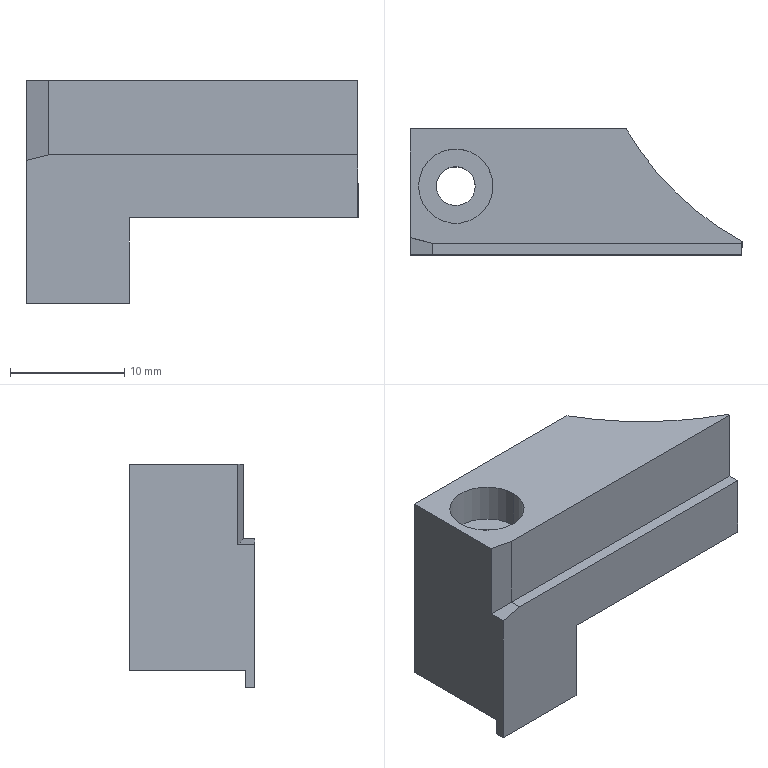Part | STEP file | 11-FG-B07111 | 1 solid | 20 faces | box 29 x 11 x 19.5 mm | volume 3288 mm3 | plane 15 | cylinder 5 | commonest cylinder face diameters 3.4 x2 6.5 x2 51 x1
STEP:
#1=CARTESIAN_POINT('',(-13.75,0.,14.6));
#2=VERTEX_POINT('',#1);
#3=CARTESIAN_POINT('',(-7.25,0.,14.6));
#4=VERTEX_POINT('',#3);
#5=CARTESIAN_POINT('',(-10.5,0.,14.6));
#6=DIRECTION('',(0.,0.,1.));
#7=DIRECTION('',(1.,0.,0.));
#8=AXIS2_PLACEMENT_3D('',#5,#6,#7);
#9=CIRCLE('',#8,3.25);
#10=EDGE_CURVE('',#2,#4,#9,.T.);
#11=ORIENTED_EDGE('',*,*,#10,.F.);
#12=CARTESIAN_POINT('',(-13.75,0.,18.));
#13=VERTEX_POINT('',#12);
#14=CARTESIAN_POINT('',(-13.75,0.,18.));
#15=DIRECTION('',(0.,0.,1.));
#16=VECTOR('',#15,1000.);
#17=LINE('',#14,#16);
#18=EDGE_CURVE('',#2,#13,#17,.T.);
#19=ORIENTED_EDGE('',*,*,#18,.T.);
#20=CARTESIAN_POINT('',(-7.25,0.,18.));
#21=VERTEX_POINT('',#20);
#22=CARTESIAN_POINT('',(-10.5,0.,18.));
#23=DIRECTION('',(0.,0.,1.));
#24=DIRECTION('',(1.,0.,0.));
#25=AXIS2_PLACEMENT_3D('',#22,#23,#24);
#26=CIRCLE('',#25,3.25);
#27=EDGE_CURVE('',#13,#21,#26,.T.);
#28=ORIENTED_EDGE('',*,*,#27,.T.);
#29=CARTESIAN_POINT('',(-7.25,0.,18.));
#30=DIRECTION('',(0.,0.,1.));
#31=VECTOR('',#30,1000.);
#32=LINE('',#29,#31);
#33=EDGE_CURVE('',#4,#21,#32,.T.);
#34=ORIENTED_EDGE('',*,*,#33,.F.);
#35=EDGE_LOOP('',(#11,#19,#28,#34));
#36=FACE_OUTER_BOUND('',#35,.T.);
#37=CARTESIAN_POINT('',(-10.5,0.,18.));
#38=DIRECTION('',(0.,0.,1.));
#39=DIRECTION('',(1.,0.,0.));
#40=AXIS2_PLACEMENT_3D('',#37,#38,#39);
#41=CYLINDRICAL_SURFACE('',#40,3.25);
#42=ADVANCED_FACE('',(#36),#41,.F.);
#43=CARTESIAN_POINT('',(-12.2,0.,0.));
#44=VERTEX_POINT('',#43);
#45=CARTESIAN_POINT('',(-8.8,0.,0.));
#46=VERTEX_POINT('',#45);
#47=CARTESIAN_POINT('',(-10.5,0.,0.));
#48=DIRECTION('',(0.,0.,1.));
#49=DIRECTION('',(1.,0.,0.));
#50=AXIS2_PLACEMENT_3D('',#47,#48,#49);
#51=CIRCLE('',#50,1.7);
#52=EDGE_CURVE('',#44,#46,#51,.T.);
#53=ORIENTED_EDGE('',*,*,#52,.F.);
#54=CARTESIAN_POINT('',(-12.2,0.,14.6));
#55=VERTEX_POINT('',#54);
#56=CARTESIAN_POINT('',(-12.2,0.,18.));
#57=DIRECTION('',(0.,0.,1.));
#58=VECTOR('',#57,1000.);
#59=LINE('',#56,#58);
#60=EDGE_CURVE('',#44,#55,#59,.T.);
#61=ORIENTED_EDGE('',*,*,#60,.T.);
#62=CARTESIAN_POINT('',(-8.8,0.,14.6));
#63=VERTEX_POINT('',#62);
#64=CARTESIAN_POINT('',(-10.5,0.,14.6));
#65=DIRECTION('',(0.,0.,1.));
#66=DIRECTION('',(1.,0.,0.));
#67=AXIS2_PLACEMENT_3D('',#64,#65,#66);
#68=CIRCLE('',#67,1.7);
#69=EDGE_CURVE('',#55,#63,#68,.T.);
#70=ORIENTED_EDGE('',*,*,#69,.T.);
#71=CARTESIAN_POINT('',(-8.8,0.,18.));
#72=DIRECTION('',(0.,0.,1.));
#73=VECTOR('',#72,1000.);
#74=LINE('',#71,#73);
#75=EDGE_CURVE('',#46,#63,#74,.T.);
#76=ORIENTED_EDGE('',*,*,#75,.F.);
#77=EDGE_LOOP('',(#53,#61,#70,#76));
#78=FACE_OUTER_BOUND('',#77,.T.);
#79=CARTESIAN_POINT('',(-10.5,0.,18.));
#80=DIRECTION('',(0.,0.,1.));
#81=DIRECTION('',(1.,0.,0.));
#82=AXIS2_PLACEMENT_3D('',#79,#80,#81);
#83=CYLINDRICAL_SURFACE('',#82,1.7);
#84=ADVANCED_FACE('',(#78),#83,.F.);
#85=CARTESIAN_POINT('',(-10.5,0.,0.));
#86=DIRECTION('',(0.,0.,1.));
#87=DIRECTION('',(1.,0.,0.));
#88=AXIS2_PLACEMENT_3D('',#85,#86,#87);
#89=CIRCLE('',#88,1.7);
#90=EDGE_CURVE('',#46,#44,#89,.T.);
#91=ORIENTED_EDGE('',*,*,#90,.T.);
#92=ORIENTED_EDGE('',*,*,#52,.T.);
#93=EDGE_LOOP('',(#91,#92));
#94=FACE_BOUND('',#93,.T.);
#95=CARTESIAN_POINT('',(-14.5,-5.2,0.));
#96=VERTEX_POINT('',#95);
#97=CARTESIAN_POINT('',(-5.5,-5.2,0.));
#98=VERTEX_POINT('',#97);
#99=CARTESIAN_POINT('',(-14.5,-5.2,0.));
#100=DIRECTION('',(1.,0.,0.));
#101=VECTOR('',#100,1000.);
#102=LINE('',#99,#101);
#103=EDGE_CURVE('',#96,#98,#102,.T.);
#104=ORIENTED_EDGE('',*,*,#103,.F.);
#105=CARTESIAN_POINT('',(-14.5,5.,0.));
#106=VERTEX_POINT('',#105);
#107=CARTESIAN_POINT('',(-14.5,-5.,0.));
#108=DIRECTION('',(0.,-1.,0.));
#109=VECTOR('',#108,1000.);
#110=LINE('',#107,#109);
#111=EDGE_CURVE('',#106,#96,#110,.T.);
#112=ORIENTED_EDGE('',*,*,#111,.F.);
#113=CARTESIAN_POINT('',(-5.5,5.,0.));
#114=VERTEX_POINT('',#113);
#115=CARTESIAN_POINT('',(14.5,5.,0.));
#116=DIRECTION('',(-1.,0.,0.));
#117=VECTOR('',#116,1000.);
#118=LINE('',#115,#117);
#119=EDGE_CURVE('',#114,#106,#118,.T.);
#120=ORIENTED_EDGE('',*,*,#119,.F.);
#121=CARTESIAN_POINT('',(-5.5,-5.,0.));
#122=DIRECTION('',(0.,1.,0.));
#123=VECTOR('',#122,1000.);
#124=LINE('',#121,#123);
#125=EDGE_CURVE('',#98,#114,#124,.T.);
#126=ORIENTED_EDGE('',*,*,#125,.F.);
#127=EDGE_LOOP('',(#104,#112,#120,#126));
#128=FACE_OUTER_BOUND('',#127,.T.);
#129=CARTESIAN_POINT('',(0.,0.,0.));
#130=DIRECTION('',(0.,0.,1.));
#131=DIRECTION('',(1.,0.,0.));
#132=AXIS2_PLACEMENT_3D('',#129,#130,#131);
#133=PLANE('',#132);
#134=ADVANCED_FACE('',(#94,#128),#133,.F.);
#135=CARTESIAN_POINT('',(-12.5,-5.,18.));
#136=VERTEX_POINT('',#135);
#137=CARTESIAN_POINT('',(14.5,-5.,18.));
#138=VERTEX_POINT('',#137);
#139=CARTESIAN_POINT('',(14.5,-5.,18.));
#140=DIRECTION('',(1.,0.,0.));
#141=VECTOR('',#140,1000.);
#142=LINE('',#139,#141);
#143=EDGE_CURVE('',#136,#138,#142,.T.);
#144=ORIENTED_EDGE('',*,*,#143,.F.);
#145=CARTESIAN_POINT('',(-12.5,-5.,11.5));
#146=VERTEX_POINT('',#145);
#147=CARTESIAN_POINT('',(-12.5,-5.,18.));
#148=DIRECTION('',(0.,0.,-1.));
#149=VECTOR('',#148,1000.);
#150=LINE('',#147,#149);
#151=EDGE_CURVE('',#136,#146,#150,.T.);
#152=ORIENTED_EDGE('',*,*,#151,.T.);
#153=CARTESIAN_POINT('',(14.5,-5.,11.5));
#154=VERTEX_POINT('',#153);
#155=CARTESIAN_POINT('',(-14.5,-5.,11.5));
#156=DIRECTION('',(-1.,0.,0.));
#157=VECTOR('',#156,1000.);
#158=LINE('',#155,#157);
#159=EDGE_CURVE('',#154,#146,#158,.T.);
#160=ORIENTED_EDGE('',*,*,#159,.F.);
#161=CARTESIAN_POINT('',(14.5,-5.,18.));
#162=DIRECTION('',(0.,0.,-1.));
#163=VECTOR('',#162,1000.);
#164=LINE('',#161,#163);
#165=EDGE_CURVE('',#138,#154,#164,.T.);
#166=ORIENTED_EDGE('',*,*,#165,.F.);
#167=EDGE_LOOP('',(#144,#152,#160,#166));
#168=FACE_OUTER_BOUND('',#167,.T.);
#169=CARTESIAN_POINT('',(14.5,-5.,18.));
#170=DIRECTION('',(0.,1.,0.));
#171=DIRECTION('',(-1.,0.,0.));
#172=AXIS2_PLACEMENT_3D('',#169,#170,#171);
#173=PLANE('',#172);
#174=ADVANCED_FACE('',(#168),#173,.F.);
#175=CARTESIAN_POINT('',(-14.5,-6.,11.));
#176=VERTEX_POINT('',#175);
#177=CARTESIAN_POINT('',(-14.5,-6.,-1.5));
#178=VERTEX_POINT('',#177);
#179=CARTESIAN_POINT('',(-14.5,-6.,0.));
#180=DIRECTION('',(0.,0.,-1.));
#181=VECTOR('',#180,1000.);
#182=LINE('',#179,#181);
#183=EDGE_CURVE('',#176,#178,#182,.T.);
#184=ORIENTED_EDGE('',*,*,#183,.F.);
#185=CARTESIAN_POINT('',(-14.5,-4.5,11.));
#186=VERTEX_POINT('',#185);
#187=CARTESIAN_POINT('',(-14.5,-5.,11.));
#188=DIRECTION('',(0.,1.,0.));
#189=VECTOR('',#188,1000.);
#190=LINE('',#187,#189);
#191=EDGE_CURVE('',#176,#186,#190,.T.);
#192=ORIENTED_EDGE('',*,*,#191,.T.);
#193=CARTESIAN_POINT('',(-14.5,-4.5,18.));
#194=VERTEX_POINT('',#193);
#195=CARTESIAN_POINT('',(-14.5,-4.5,18.));
#196=DIRECTION('',(0.,0.,1.));
#197=VECTOR('',#196,1000.);
#198=LINE('',#195,#197);
#199=EDGE_CURVE('',#186,#194,#198,.T.);
#200=ORIENTED_EDGE('',*,*,#199,.T.);
#201=CARTESIAN_POINT('',(-14.5,5.,18.));
#202=VERTEX_POINT('',#201);
#203=CARTESIAN_POINT('',(-14.5,-5.,18.));
#204=DIRECTION('',(0.,-1.,0.));
#205=VECTOR('',#204,1000.);
#206=LINE('',#203,#205);
#207=EDGE_CURVE('',#202,#194,#206,.T.);
#208=ORIENTED_EDGE('',*,*,#207,.F.);
#209=CARTESIAN_POINT('',(-14.5,5.,18.));
#210=DIRECTION('',(0.,0.,-1.));
#211=VECTOR('',#210,1000.);
#212=LINE('',#209,#211);
#213=EDGE_CURVE('',#202,#106,#212,.T.);
#214=ORIENTED_EDGE('',*,*,#213,.T.);
#215=ORIENTED_EDGE('',*,*,#111,.T.);
#216=CARTESIAN_POINT('',(-14.5,-5.2,-1.5));
#217=VERTEX_POINT('',#216);
#218=CARTESIAN_POINT('',(-14.5,-5.2,-1.5));
#219=DIRECTION('',(0.,0.,1.));
#220=VECTOR('',#219,1000.);
#221=LINE('',#218,#220);
#222=EDGE_CURVE('',#217,#96,#221,.T.);
#223=ORIENTED_EDGE('',*,*,#222,.F.);
#224=CARTESIAN_POINT('',(-14.5,-6.,-1.5));
#225=DIRECTION('',(0.,1.,0.));
#226=VECTOR('',#225,1000.);
#227=LINE('',#224,#226);
#228=EDGE_CURVE('',#178,#217,#227,.T.);
#229=ORIENTED_EDGE('',*,*,#228,.F.);
#230=EDGE_LOOP('',(#184,#192,#200,#208,#214,#215,#223,#229));
#231=FACE_OUTER_BOUND('',#230,.T.);
#232=CARTESIAN_POINT('',(-14.5,-5.,18.));
#233=DIRECTION('',(1.,0.,0.));
#234=DIRECTION('',(0.,0.,-1.));
#235=AXIS2_PLACEMENT_3D('',#232,#233,#234);
#236=PLANE('',#235);
#237=ADVANCED_FACE('',(#231),#236,.F.);
#238=CARTESIAN_POINT('',(14.5,-6.,6.));
#239=VERTEX_POINT('',#238);
#240=CARTESIAN_POINT('',(14.5,-4.8,6.));
#241=VERTEX_POINT('',#240);
#242=CARTESIAN_POINT('',(14.5,-5.,6.));
#243=DIRECTION('',(0.,1.,0.));
#244=VECTOR('',#243,1000.);
#245=LINE('',#242,#244);
#246=EDGE_CURVE('',#239,#241,#245,.T.);
#247=ORIENTED_EDGE('',*,*,#246,.T.);
#248=CARTESIAN_POINT('',(14.5,-4.8,18.));
#249=VERTEX_POINT('',#248);
#250=CARTESIAN_POINT('',(14.5,-4.8,0.));
#251=DIRECTION('',(0.,0.,1.));
#252=VECTOR('',#251,1000.);
#253=LINE('',#250,#252);
#254=EDGE_CURVE('',#241,#249,#253,.T.);
#255=ORIENTED_EDGE('',*,*,#254,.T.);
#256=CARTESIAN_POINT('',(14.5,-5.,18.));
#257=DIRECTION('',(0.,1.,0.));
#258=VECTOR('',#257,1000.);
#259=LINE('',#256,#258);
#260=EDGE_CURVE('',#138,#249,#259,.T.);
#261=ORIENTED_EDGE('',*,*,#260,.F.);
#262=ORIENTED_EDGE('',*,*,#165,.T.);
#263=CARTESIAN_POINT('',(14.5,-6.,11.5));
#264=VERTEX_POINT('',#263);
#265=CARTESIAN_POINT('',(14.5,-6.,11.5));
#266=DIRECTION('',(0.,1.,0.));
#267=VECTOR('',#266,1000.);
#268=LINE('',#265,#267);
#269=EDGE_CURVE('',#264,#154,#268,.T.);
#270=ORIENTED_EDGE('',*,*,#269,.F.);
#271=CARTESIAN_POINT('',(14.5,-6.,6.));
#272=DIRECTION('',(0.,0.,1.));
#273=VECTOR('',#272,1000.);
#274=LINE('',#271,#273);
#275=EDGE_CURVE('',#239,#264,#274,.T.);
#276=ORIENTED_EDGE('',*,*,#275,.F.);
#277=EDGE_LOOP('',(#247,#255,#261,#262,#270,#276));
#278=FACE_OUTER_BOUND('',#277,.T.);
#279=CARTESIAN_POINT('',(14.5,-5.,18.));
#280=DIRECTION('',(-1.,0.,0.));
#281=DIRECTION('',(0.,0.,1.));
#282=AXIS2_PLACEMENT_3D('',#279,#280,#281);
#283=PLANE('',#282);
#284=ADVANCED_FACE('',(#278),#283,.F.);
#285=CARTESIAN_POINT('',(4.388,5.,18.));
#286=VERTEX_POINT('',#285);
#287=CARTESIAN_POINT('',(14.5,5.,18.));
#288=DIRECTION('',(-1.,0.,0.));
#289=VECTOR('',#288,1000.);
#290=LINE('',#287,#289);
#291=EDGE_CURVE('',#286,#202,#290,.T.);
#292=ORIENTED_EDGE('',*,*,#291,.F.);
#293=CARTESIAN_POINT('',(4.388,5.,6.));
#294=VERTEX_POINT('',#293);
#295=CARTESIAN_POINT('',(4.388,5.,0.));
#296=DIRECTION('',(0.,0.,-1.));
#297=VECTOR('',#296,1000.);
#298=LINE('',#295,#297);
#299=EDGE_CURVE('',#286,#294,#298,.T.);
#300=ORIENTED_EDGE('',*,*,#299,.T.);
#301=CARTESIAN_POINT('',(-5.5,5.,6.));
#302=VERTEX_POINT('',#301);
#303=CARTESIAN_POINT('',(-5.5,5.,6.));
#304=DIRECTION('',(1.,0.,0.));
#305=VECTOR('',#304,1000.);
#306=LINE('',#303,#305);
#307=EDGE_CURVE('',#302,#294,#306,.T.);
#308=ORIENTED_EDGE('',*,*,#307,.F.);
#309=CARTESIAN_POINT('',(-5.5,5.,0.));
#310=DIRECTION('',(0.,0.,1.));
#311=VECTOR('',#310,1000.);
#312=LINE('',#309,#311);
#313=EDGE_CURVE('',#114,#302,#312,.T.);
#314=ORIENTED_EDGE('',*,*,#313,.F.);
#315=ORIENTED_EDGE('',*,*,#119,.T.);
#316=ORIENTED_EDGE('',*,*,#213,.F.);
#317=EDGE_LOOP('',(#292,#300,#308,#314,#315,#316));
#318=FACE_OUTER_BOUND('',#317,.T.);
#319=CARTESIAN_POINT('',(14.5,5.,18.));
#320=DIRECTION('',(0.,-1.,0.));
#321=DIRECTION('',(1.,0.,0.));
#322=AXIS2_PLACEMENT_3D('',#319,#320,#321);
#323=PLANE('',#322);
#324=ADVANCED_FACE('',(#318),#323,.F.);
#325=ORIENTED_EDGE('',*,*,#207,.T.);
#326=CARTESIAN_POINT('',(-1.912,-7.647,18.));
#327=DIRECTION('',(0.9701,-0.2425,0.));
#328=VECTOR('',#327,1000.);
#329=LINE('',#326,#328);
#330=EDGE_CURVE('',#194,#136,#329,.T.);
#331=ORIENTED_EDGE('',*,*,#330,.T.);
#332=ORIENTED_EDGE('',*,*,#143,.T.);
#333=ORIENTED_EDGE('',*,*,#260,.T.);
#334=CARTESIAN_POINT('',(26.5,17.7,18.));
#335=DIRECTION('',(0.,0.,1.));
#336=DIRECTION('',(1.,0.,0.));
#337=AXIS2_PLACEMENT_3D('',#334,#335,#336);
#338=CIRCLE('',#337,25.5);
#339=EDGE_CURVE('',#286,#249,#338,.T.);
#340=ORIENTED_EDGE('',*,*,#339,.F.);
#341=ORIENTED_EDGE('',*,*,#291,.T.);
#342=EDGE_LOOP('',(#325,#331,#332,#333,#340,#341));
#343=FACE_OUTER_BOUND('',#342,.T.);
#344=CARTESIAN_POINT('',(-10.5,0.,18.));
#345=DIRECTION('',(0.,0.,1.));
#346=DIRECTION('',(1.,0.,0.));
#347=AXIS2_PLACEMENT_3D('',#344,#345,#346);
#348=CIRCLE('',#347,3.25);
#349=EDGE_CURVE('',#21,#13,#348,.T.);
#350=ORIENTED_EDGE('',*,*,#349,.F.);
#351=ORIENTED_EDGE('',*,*,#27,.F.);
#352=EDGE_LOOP('',(#350,#351));
#353=FACE_BOUND('',#352,.T.);
#354=CARTESIAN_POINT('',(0.,0.,18.));
#355=DIRECTION('',(0.,0.,1.));
#356=DIRECTION('',(1.,0.,0.));
#357=AXIS2_PLACEMENT_3D('',#354,#355,#356);
#358=PLANE('',#357);
#359=ADVANCED_FACE('',(#343,#353),#358,.T.);
#360=ORIENTED_EDGE('',*,*,#313,.T.);
#361=CARTESIAN_POINT('',(-5.5,-6.,6.));
#362=VERTEX_POINT('',#361);
#363=CARTESIAN_POINT('',(-5.5,-5.,6.));
#364=DIRECTION('',(0.,1.,0.));
#365=VECTOR('',#364,1000.);
#366=LINE('',#363,#365);
#367=EDGE_CURVE('',#362,#302,#366,.T.);
#368=ORIENTED_EDGE('',*,*,#367,.F.);
#369=CARTESIAN_POINT('',(-5.5,-6.,-1.5));
#370=VERTEX_POINT('',#369);
#371=CARTESIAN_POINT('',(-5.5,-6.,6.));
#372=DIRECTION('',(0.,0.,1.));
#373=VECTOR('',#372,1000.);
#374=LINE('',#371,#373);
#375=EDGE_CURVE('',#370,#362,#374,.T.);
#376=ORIENTED_EDGE('',*,*,#375,.F.);
#377=CARTESIAN_POINT('',(-5.5,-5.2,-1.5));
#378=VERTEX_POINT('',#377);
#379=CARTESIAN_POINT('',(-5.5,-6.,-1.5));
#380=DIRECTION('',(0.,-1.,0.));
#381=VECTOR('',#380,1000.);
#382=LINE('',#379,#381);
#383=EDGE_CURVE('',#378,#370,#382,.T.);
#384=ORIENTED_EDGE('',*,*,#383,.F.);
#385=CARTESIAN_POINT('',(-5.5,-5.2,-1.5));
#386=DIRECTION('',(0.,0.,1.));
#387=VECTOR('',#386,1000.);
#388=LINE('',#385,#387);
#389=EDGE_CURVE('',#378,#98,#388,.T.);
#390=ORIENTED_EDGE('',*,*,#389,.T.);
#391=ORIENTED_EDGE('',*,*,#125,.T.);
#392=EDGE_LOOP('',(#360,#368,#376,#384,#390,#391));
#393=FACE_OUTER_BOUND('',#392,.T.);
#394=CARTESIAN_POINT('',(-5.5,-5.,0.));
#395=DIRECTION('',(-1.,0.,0.));
#396=DIRECTION('',(0.,-1.,0.));
#397=AXIS2_PLACEMENT_3D('',#394,#395,#396);
#398=PLANE('',#397);
#399=ADVANCED_FACE('',(#393),#398,.F.);
#400=ORIENTED_EDGE('',*,*,#307,.T.);
#401=CARTESIAN_POINT('',(26.5,17.7,6.));
#402=DIRECTION('',(0.,0.,1.));
#403=DIRECTION('',(1.,0.,0.));
#404=AXIS2_PLACEMENT_3D('',#401,#402,#403);
#405=CIRCLE('',#404,25.5);
#406=EDGE_CURVE('',#294,#241,#405,.T.);
#407=ORIENTED_EDGE('',*,*,#406,.T.);
#408=ORIENTED_EDGE('',*,*,#246,.F.);
#409=CARTESIAN_POINT('',(-5.5,-6.,6.));
#410=DIRECTION('',(1.,0.,0.));
#411=VECTOR('',#410,1000.);
#412=LINE('',#409,#411);
#413=EDGE_CURVE('',#362,#239,#412,.T.);
#414=ORIENTED_EDGE('',*,*,#413,.F.);
#415=ORIENTED_EDGE('',*,*,#367,.T.);
#416=EDGE_LOOP('',(#400,#407,#408,#414,#415));
#417=FACE_OUTER_BOUND('',#416,.T.);
#418=CARTESIAN_POINT('',(-5.5,-5.,6.));
#419=DIRECTION('',(0.,0.,1.));
#420=DIRECTION('',(1.,0.,0.));
#421=AXIS2_PLACEMENT_3D('',#418,#419,#420);
#422=PLANE('',#421);
#423=ADVANCED_FACE('',(#417),#422,.F.);
#424=ORIENTED_EDGE('',*,*,#60,.F.);
#425=ORIENTED_EDGE('',*,*,#90,.F.);
#426=ORIENTED_EDGE('',*,*,#75,.T.);
#427=CARTESIAN_POINT('',(-10.5,0.,14.6));
#428=DIRECTION('',(0.,0.,1.));
#429=DIRECTION('',(1.,0.,0.));
#430=AXIS2_PLACEMENT_3D('',#427,#428,#429);
#431=CIRCLE('',#430,1.7);
#432=EDGE_CURVE('',#63,#55,#431,.T.);
#433=ORIENTED_EDGE('',*,*,#432,.T.);
#434=EDGE_LOOP('',(#424,#425,#426,#433));
#435=FACE_OUTER_BOUND('',#434,.T.);
#436=CARTESIAN_POINT('',(-10.5,0.,18.));
#437=DIRECTION('',(0.,0.,1.));
#438=DIRECTION('',(1.,0.,0.));
#439=AXIS2_PLACEMENT_3D('',#436,#437,#438);
#440=CYLINDRICAL_SURFACE('',#439,1.7);
#441=ADVANCED_FACE('',(#435),#440,.F.);
#442=ORIENTED_EDGE('',*,*,#432,.F.);
#443=ORIENTED_EDGE('',*,*,#69,.F.);
#444=EDGE_LOOP('',(#442,#443));
#445=FACE_BOUND('',#444,.T.);
#446=CARTESIAN_POINT('',(-10.5,0.,14.6));
#447=DIRECTION('',(0.,0.,1.));
#448=DIRECTION('',(1.,0.,0.));
#449=AXIS2_PLACEMENT_3D('',#446,#447,#448);
#450=CIRCLE('',#449,3.25);
#451=EDGE_CURVE('',#4,#2,#450,.T.);
#452=ORIENTED_EDGE('',*,*,#451,.T.);
#453=ORIENTED_EDGE('',*,*,#10,.T.);
#454=EDGE_LOOP('',(#452,#453));
#455=FACE_OUTER_BOUND('',#454,.T.);
#456=CARTESIAN_POINT('',(-8.8,0.,14.6));
#457=DIRECTION('',(0.,0.,-1.));
#458=DIRECTION('',(-1.,0.,0.));
#459=AXIS2_PLACEMENT_3D('',#456,#457,#458);
#460=PLANE('',#459);
#461=ADVANCED_FACE('',(#445,#455),#460,.F.);
#462=ORIENTED_EDGE('',*,*,#18,.F.);
#463=ORIENTED_EDGE('',*,*,#451,.F.);
#464=ORIENTED_EDGE('',*,*,#33,.T.);
#465=ORIENTED_EDGE('',*,*,#349,.T.);
#466=EDGE_LOOP('',(#462,#463,#464,#465));
#467=FACE_OUTER_BOUND('',#466,.T.);
#468=CARTESIAN_POINT('',(-10.5,0.,18.));
#469=DIRECTION('',(0.,0.,1.));
#470=DIRECTION('',(1.,0.,0.));
#471=AXIS2_PLACEMENT_3D('',#468,#469,#470);
#472=CYLINDRICAL_SURFACE('',#471,3.25);
#473=ADVANCED_FACE('',(#467),#472,.F.);
#474=ORIENTED_EDGE('',*,*,#406,.F.);
#475=ORIENTED_EDGE('',*,*,#299,.F.);
#476=ORIENTED_EDGE('',*,*,#339,.T.);
#477=ORIENTED_EDGE('',*,*,#254,.F.);
#478=EDGE_LOOP('',(#474,#475,#476,#477));
#479=FACE_OUTER_BOUND('',#478,.T.);
#480=CARTESIAN_POINT('',(26.5,17.7,0.));
#481=DIRECTION('',(0.,0.,1.));
#482=DIRECTION('',(1.,0.,0.));
#483=AXIS2_PLACEMENT_3D('',#480,#481,#482);
#484=CYLINDRICAL_SURFACE('',#483,25.5);
#485=ADVANCED_FACE('',(#479),#484,.F.);
#486=ORIENTED_EDGE('',*,*,#159,.T.);
#487=CARTESIAN_POINT('',(-12.5,-6.,11.5));
#488=VERTEX_POINT('',#487);
#489=CARTESIAN_POINT('',(-12.5,-6.,11.5));
#490=DIRECTION('',(0.,-1.,0.));
#491=VECTOR('',#490,1000.);
#492=LINE('',#489,#491);
#493=EDGE_CURVE('',#146,#488,#492,.T.);
#494=ORIENTED_EDGE('',*,*,#493,.T.);
#495=CARTESIAN_POINT('',(-14.5,-6.,11.5));
#496=DIRECTION('',(-1.,0.,0.));
#497=VECTOR('',#496,1000.);
#498=LINE('',#495,#497);
#499=EDGE_CURVE('',#264,#488,#498,.T.);
#500=ORIENTED_EDGE('',*,*,#499,.F.);
#501=ORIENTED_EDGE('',*,*,#269,.T.);
#502=EDGE_LOOP('',(#486,#494,#500,#501));
#503=FACE_OUTER_BOUND('',#502,.T.);
#504=CARTESIAN_POINT('',(-14.5,-6.,11.5));
#505=DIRECTION('',(0.,0.,-1.));
#506=DIRECTION('',(-1.,0.,0.));
#507=AXIS2_PLACEMENT_3D('',#504,#505,#506);
#508=PLANE('',#507);
#509=ADVANCED_FACE('',(#503),#508,.F.);
#510=ORIENTED_EDGE('',*,*,#499,.T.);
#511=CARTESIAN_POINT('',(-14.5,-6.,11.));
#512=DIRECTION('',(-0.9701,0.,-0.2425));
#513=VECTOR('',#512,1000.);
#514=LINE('',#511,#513);
#515=EDGE_CURVE('',#488,#176,#514,.T.);
#516=ORIENTED_EDGE('',*,*,#515,.T.);
#517=ORIENTED_EDGE('',*,*,#183,.T.);
#518=CARTESIAN_POINT('',(-14.5,-6.,-1.5));
#519=DIRECTION('',(-1.,0.,0.));
#520=VECTOR('',#519,1000.);
#521=LINE('',#518,#520);
#522=EDGE_CURVE('',#370,#178,#521,.T.);
#523=ORIENTED_EDGE('',*,*,#522,.F.);
#524=ORIENTED_EDGE('',*,*,#375,.T.);
#525=ORIENTED_EDGE('',*,*,#413,.T.);
#526=ORIENTED_EDGE('',*,*,#275,.T.);
#527=EDGE_LOOP('',(#510,#516,#517,#523,#524,#525,#526));
#528=FACE_OUTER_BOUND('',#527,.T.);
#529=CARTESIAN_POINT('',(0.,-6.,0.));
#530=DIRECTION('',(0.,1.,0.));
#531=DIRECTION('',(-1.,0.,0.));
#532=AXIS2_PLACEMENT_3D('',#529,#530,#531);
#533=PLANE('',#532);
#534=ADVANCED_FACE('',(#528),#533,.F.);
#535=ORIENTED_EDGE('',*,*,#330,.F.);
#536=ORIENTED_EDGE('',*,*,#199,.F.);
#537=CARTESIAN_POINT('',(-14.389,-4.528,11.028));
#538=DIRECTION('',(-0.9428,0.2357,-0.2357));
#539=VECTOR('',#538,1000.);
#540=LINE('',#537,#539);
#541=EDGE_CURVE('',#146,#186,#540,.T.);
#542=ORIENTED_EDGE('',*,*,#541,.F.);
#543=ORIENTED_EDGE('',*,*,#151,.F.);
#544=EDGE_LOOP('',(#535,#536,#542,#543));
#545=FACE_OUTER_BOUND('',#544,.T.);
#546=CARTESIAN_POINT('',(-12.5,-5.,18.));
#547=DIRECTION('',(0.2425,0.9701,0.));
#548=DIRECTION('',(0.,0.,-1.));
#549=AXIS2_PLACEMENT_3D('',#546,#547,#548);
#550=PLANE('',#549);
#551=ADVANCED_FACE('',(#545),#550,.F.);
#552=ORIENTED_EDGE('',*,*,#515,.F.);
#553=ORIENTED_EDGE('',*,*,#493,.F.);
#554=ORIENTED_EDGE('',*,*,#541,.T.);
#555=ORIENTED_EDGE('',*,*,#191,.F.);
#556=EDGE_LOOP('',(#552,#553,#554,#555));
#557=FACE_OUTER_BOUND('',#556,.T.);
#558=CARTESIAN_POINT('',(-14.5,-5.,11.));
#559=DIRECTION('',(0.2425,0.,-0.9701));
#560=DIRECTION('',(0.,1.,0.));
#561=AXIS2_PLACEMENT_3D('',#558,#559,#560);
#562=PLANE('',#561);
#563=ADVANCED_FACE('',(#557),#562,.F.);
#564=ORIENTED_EDGE('',*,*,#103,.T.);
#565=ORIENTED_EDGE('',*,*,#389,.F.);
#566=CARTESIAN_POINT('',(-14.5,-5.2,-1.5));
#567=DIRECTION('',(1.,0.,0.));
#568=VECTOR('',#567,1000.);
#569=LINE('',#566,#568);
#570=EDGE_CURVE('',#217,#378,#569,.T.);
#571=ORIENTED_EDGE('',*,*,#570,.F.);
#572=ORIENTED_EDGE('',*,*,#222,.T.);
#573=EDGE_LOOP('',(#564,#565,#571,#572));
#574=FACE_OUTER_BOUND('',#573,.T.);
#575=CARTESIAN_POINT('',(-14.5,-5.2,-1.5));
#576=DIRECTION('',(0.,-1.,0.));
#577=DIRECTION('',(0.,0.,-1.));
#578=AXIS2_PLACEMENT_3D('',#575,#576,#577);
#579=PLANE('',#578);
#580=ADVANCED_FACE('',(#574),#579,.F.);
#581=ORIENTED_EDGE('',*,*,#228,.T.);
#582=ORIENTED_EDGE('',*,*,#570,.T.);
#583=ORIENTED_EDGE('',*,*,#383,.T.);
#584=ORIENTED_EDGE('',*,*,#522,.T.);
#585=EDGE_LOOP('',(#581,#582,#583,#584));
#586=FACE_OUTER_BOUND('',#585,.T.);
#587=CARTESIAN_POINT('',(0.,0.,-1.5));
#588=DIRECTION('',(0.,0.,-1.));
#589=DIRECTION('',(-1.,0.,0.));
#590=AXIS2_PLACEMENT_3D('',#587,#588,#589);
#591=PLANE('',#590);
#592=ADVANCED_FACE('',(#586),#591,.T.);
#593=CLOSED_SHELL('',(#42,#84,#134,#174,#237,#284,#324,#359,#399,#423,#441,#461,#473,#485,#509,#534,#551,#563,#580,#592));
#594=MANIFOLD_SOLID_BREP('',#593);
#595=CARTESIAN_POINT('',(0.,0.,0.));
#596=DIRECTION('',(0.,0.,1.));
#597=DIRECTION('',(1.,0.,0.));
#598=AXIS2_PLACEMENT_3D('',#595,#596,#597);
#599=(LENGTH_UNIT()NAMED_UNIT(*)SI_UNIT(.MILLI.,.METRE.));
#600=UNCERTAINTY_MEASURE_WITH_UNIT(LENGTH_MEASURE(0.00001),#599,'','');
#601=(NAMED_UNIT(*)PLANE_ANGLE_UNIT()SI_UNIT($,.RADIAN.));
#602=(NAMED_UNIT(*)SI_UNIT($,.STERADIAN.)SOLID_ANGLE_UNIT());
#603=(GEOMETRIC_REPRESENTATION_CONTEXT(3)GLOBAL_UNCERTAINTY_ASSIGNED_CONTEXT((#600))GLOBAL_UNIT_ASSIGNED_CONTEXT((#599,#601,#602))REPRESENTATION_CONTEXT('',''));
#604=ADVANCED_BREP_SHAPE_REPRESENTATION('',(#594,#598),#603);